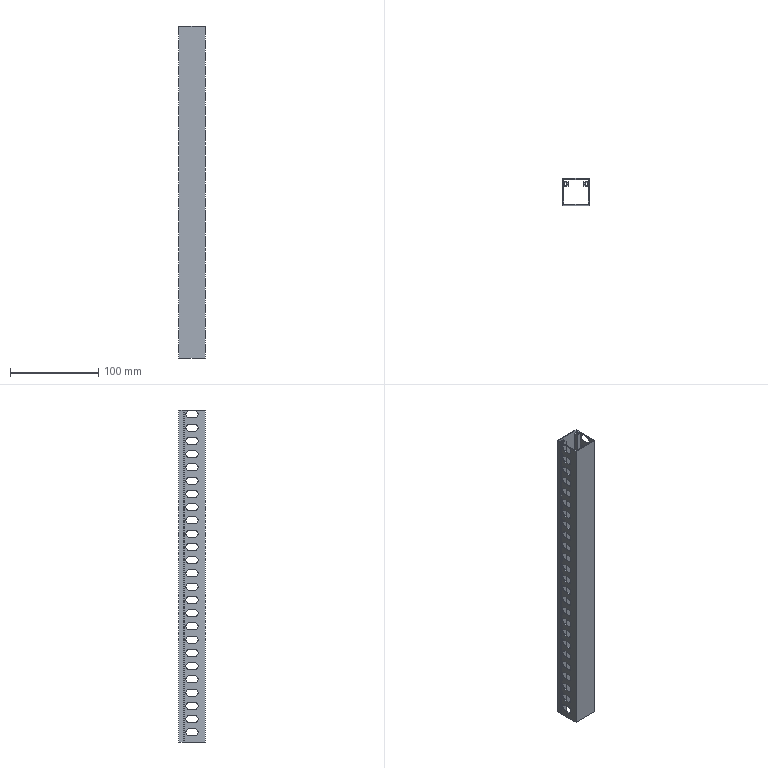Part | SolidWorks | features BaseBody 1 | 1 solid | 226 faces | box 30 x 30 x 375.9 mm | volume 46209 mm3 | plane 126 | cylinder 100 | commonest cylinder face diameters 8 x100